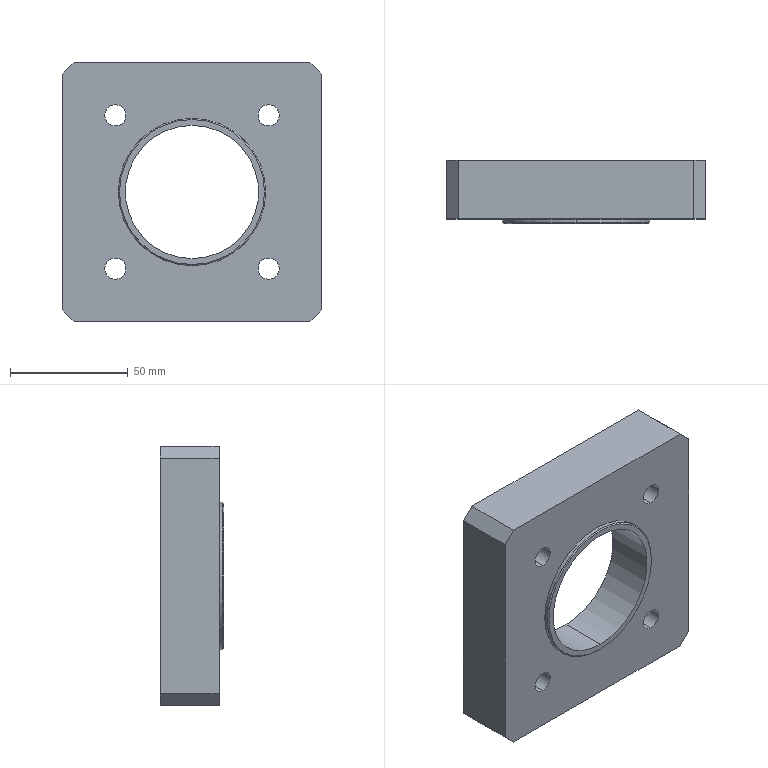Part | SolidWorks | features Chamfer 3, ICE 3, HoleWzd 2, Extrusion 1 | 1 solid | 64 faces | box 110 x 27 x 110 mm | volume 202439 mm3 | cylinder 33 | plane 16 | cone 15 | commonest cylinder face diameters 6.8 x8 9 x8 15 x8 85 x5 56.5 x2 62.5 x2